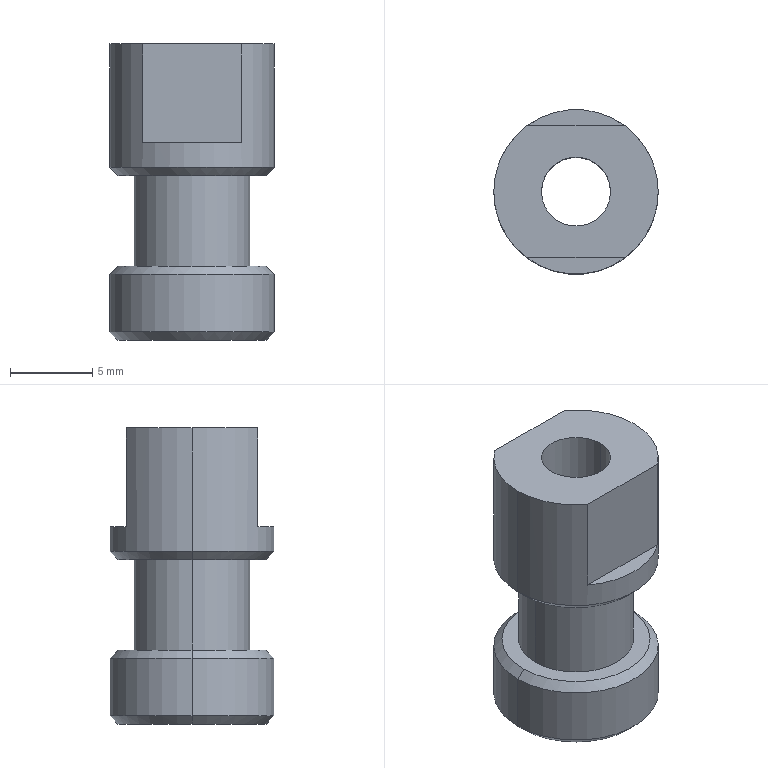Part | STEP file | PN_0051 Mount electronic clip movable connector head | 1 solid | 22 faces | box 10 x 10 x 18 mm | volume 883.594 mm3 | cylinder 8 | plane 8 | cone 6 | commonest cylinder face diameters 10 x4 4.2 x2 7 x2
STEP:
#1=CARTESIAN_POINT('',(0.,0.,0.));
#2=DIRECTION('',(0.,0.,1.));
#3=DIRECTION('',(1.,0.,0.));
#4=AXIS2_PLACEMENT_3D('',#1,#2,#3);
#5=CARTESIAN_POINT('',(-4.5,0.,0.));
#6=VERTEX_POINT('',#5);
#7=CARTESIAN_POINT('',(4.5,0.,0.));
#8=VERTEX_POINT('',#7);
#9=CARTESIAN_POINT('',(0.,0.,0.));
#10=DIRECTION('',(0.,0.,-1.));
#11=DIRECTION('',(1.,0.,0.));
#12=AXIS2_PLACEMENT_3D('',#9,#10,#11);
#13=CIRCLE('',#12,4.5);
#14=CARTESIAN_POINT('',(0.,0.,0.5));
#15=DIRECTION('',(0.,0.,1.));
#16=DIRECTION('',(1.,0.,0.));
#17=AXIS2_PLACEMENT_3D('',#14,#15,#16);
#18=CONICAL_SURFACE('',#17,5.,0.7854);
#19=CARTESIAN_POINT('',(6.283,-0.5));
#20=DIRECTION('',(-1.,0.));
#21=VECTOR('',#20,1.);
#22=LINE('',#19,#21);
#23=(GEOMETRIC_REPRESENTATION_CONTEXT(2)PARAMETRIC_REPRESENTATION_CONTEXT()REPRESENTATION_CONTEXT('',''));
#24=DEFINITIONAL_REPRESENTATION('',(#22),#23);
#25=PCURVE('',#18,#24);
#26=CARTESIAN_POINT('',(0.,0.,0.));
#27=DIRECTION('',(0.,0.,1.));
#28=DIRECTION('',(1.,0.,0.));
#29=AXIS2_PLACEMENT_3D('',#26,#27,#28);
#30=PLANE('',#29);
#31=CARTESIAN_POINT('',(4.5,0.));
#32=CARTESIAN_POINT('',(4.5,-7.794));
#33=CARTESIAN_POINT('',(-2.25,-3.897));
#34=CARTESIAN_POINT('',(-9.,0.));
#35=CARTESIAN_POINT('',(-2.25,3.897));
#36=CARTESIAN_POINT('',(4.5,7.794));
#37=CARTESIAN_POINT('',(4.5,0.));
#38=(BOUNDED_CURVE()B_SPLINE_CURVE(2,(#31,#32,#33,#34,#35,#36,#37),.UNSPECIFIED.,.T.,.F.)B_SPLINE_CURVE_WITH_KNOTS((1,2,2,2,2,1),(-2.094,0.,2.094,4.189,6.283,8.378),.UNSPECIFIED.)CURVE()GEOMETRIC_REPRESENTATION_ITEM()RATIONAL_B_SPLINE_CURVE((1.,0.5,1.,0.5,1.,0.5,1.))REPRESENTATION_ITEM(''));
#39=(GEOMETRIC_REPRESENTATION_CONTEXT(2)PARAMETRIC_REPRESENTATION_CONTEXT()REPRESENTATION_CONTEXT('',''));
#40=DEFINITIONAL_REPRESENTATION('',(#38),#39);
#41=PCURVE('',#30,#40);
#42=SURFACE_CURVE('',#13,(#25,#41),.PCURVE_S1.);
#43=EDGE_CURVE('',#6,#8,#42,.T.);
#44=ORIENTED_EDGE('',*,*,#43,.F.);
#45=CARTESIAN_POINT('',(-5.,0.,0.5));
#46=VERTEX_POINT('',#45);
#47=CARTESIAN_POINT('',(-5.,0.,0.5));
#48=DIRECTION('',(-0.7071,0.,0.7071));
#49=VECTOR('',#48,1.);
#50=LINE('',#47,#49);
#51=CARTESIAN_POINT('',(3.142,0.));
#52=DIRECTION('',(0.,1.));
#53=VECTOR('',#52,1.);
#54=LINE('',#51,#53);
#55=(GEOMETRIC_REPRESENTATION_CONTEXT(2)PARAMETRIC_REPRESENTATION_CONTEXT()REPRESENTATION_CONTEXT('',''));
#56=DEFINITIONAL_REPRESENTATION('',(#54),#55);
#57=PCURVE('',#18,#56);
#58=CARTESIAN_POINT('',(0.,0.,0.5));
#59=DIRECTION('',(0.,0.,1.));
#60=DIRECTION('',(1.,0.,0.));
#61=AXIS2_PLACEMENT_3D('',#58,#59,#60);
#62=CONICAL_SURFACE('',#61,5.,0.7854);
#63=CARTESIAN_POINT('',(3.142,0.));
#64=DIRECTION('',(0.,1.));
#65=VECTOR('',#64,1.);
#66=LINE('',#63,#65);
#67=(GEOMETRIC_REPRESENTATION_CONTEXT(2)PARAMETRIC_REPRESENTATION_CONTEXT()REPRESENTATION_CONTEXT('',''));
#68=DEFINITIONAL_REPRESENTATION('',(#66),#67);
#69=PCURVE('',#62,#68);
#70=SURFACE_CURVE('',#50,(#57,#69),.PCURVE_S1.);
#71=EDGE_CURVE('',#6,#46,#70,.T.);
#72=ORIENTED_EDGE('',*,*,#71,.T.);
#73=CARTESIAN_POINT('',(5.,0.,0.5));
#74=VERTEX_POINT('',#73);
#75=CARTESIAN_POINT('',(0.,0.,0.5));
#76=DIRECTION('',(0.,0.,1.));
#77=DIRECTION('',(1.,0.,0.));
#78=AXIS2_PLACEMENT_3D('',#75,#76,#77);
#79=CIRCLE('',#78,5.);
#80=CARTESIAN_POINT('',(0.,0.));
#81=DIRECTION('',(1.,0.));
#82=VECTOR('',#81,1.);
#83=LINE('',#80,#82);
#84=(GEOMETRIC_REPRESENTATION_CONTEXT(2)PARAMETRIC_REPRESENTATION_CONTEXT()REPRESENTATION_CONTEXT('',''));
#85=DEFINITIONAL_REPRESENTATION('',(#83),#84);
#86=PCURVE('',#18,#85);
#87=CARTESIAN_POINT('',(0.,0.,4.5));
#88=DIRECTION('',(0.,0.,-1.));
#89=DIRECTION('',(-1.,0.,0.));
#90=AXIS2_PLACEMENT_3D('',#87,#88,#89);
#91=CYLINDRICAL_SURFACE('',#90,5.);
#92=CARTESIAN_POINT('',(3.142,4.));
#93=DIRECTION('',(-1.,0.));
#94=VECTOR('',#93,1.);
#95=LINE('',#92,#94);
#96=(GEOMETRIC_REPRESENTATION_CONTEXT(2)PARAMETRIC_REPRESENTATION_CONTEXT()REPRESENTATION_CONTEXT('',''));
#97=DEFINITIONAL_REPRESENTATION('',(#95),#96);
#98=PCURVE('',#91,#97);
#99=SURFACE_CURVE('',#79,(#86,#98),.PCURVE_S1.);
#100=EDGE_CURVE('',#74,#46,#99,.T.);
#101=ORIENTED_EDGE('',*,*,#100,.F.);
#102=CARTESIAN_POINT('',(5.,0.,0.5));
#103=DIRECTION('',(0.7071,0.,0.7071));
#104=VECTOR('',#103,1.);
#105=LINE('',#102,#104);
#106=CARTESIAN_POINT('',(0.,0.));
#107=DIRECTION('',(0.,1.));
#108=VECTOR('',#107,1.);
#109=LINE('',#106,#108);
#110=(GEOMETRIC_REPRESENTATION_CONTEXT(2)PARAMETRIC_REPRESENTATION_CONTEXT()REPRESENTATION_CONTEXT('',''));
#111=DEFINITIONAL_REPRESENTATION('',(#109),#110);
#112=PCURVE('',#18,#111);
#113=CARTESIAN_POINT('',(6.283,0.));
#114=DIRECTION('',(0.,1.));
#115=VECTOR('',#114,1.);
#116=LINE('',#113,#115);
#117=(GEOMETRIC_REPRESENTATION_CONTEXT(2)PARAMETRIC_REPRESENTATION_CONTEXT()REPRESENTATION_CONTEXT('',''));
#118=DEFINITIONAL_REPRESENTATION('',(#116),#117);
#119=PCURVE('',#62,#118);
#120=SURFACE_CURVE('',#105,(#112,#119),.PCURVE_S1.);
#121=EDGE_CURVE('',#8,#74,#120,.T.);
#122=ORIENTED_EDGE('',*,*,#121,.F.);
#123=EDGE_LOOP('',(#44,#72,#101,#122));
#124=FACE_BOUND('',#123,.T.);
#125=ADVANCED_FACE('',(#124),#18,.T.);
#126=CARTESIAN_POINT('',(4.5,0.,4.5));
#127=VERTEX_POINT('',#126);
#128=CARTESIAN_POINT('',(-4.5,0.,4.5));
#129=VERTEX_POINT('',#128);
#130=CARTESIAN_POINT('',(0.,0.,4.5));
#131=DIRECTION('',(0.,0.,1.));
#132=DIRECTION('',(1.,0.,0.));
#133=AXIS2_PLACEMENT_3D('',#130,#131,#132);
#134=CIRCLE('',#133,4.5);
#135=CARTESIAN_POINT('',(0.,0.,4.5));
#136=DIRECTION('',(0.,0.,-1.));
#137=DIRECTION('',(-1.,0.,0.));
#138=AXIS2_PLACEMENT_3D('',#135,#136,#137);
#139=CONICAL_SURFACE('',#138,4.5,0.7854);
#140=CARTESIAN_POINT('',(3.142,0.));
#141=DIRECTION('',(-1.,0.));
#142=VECTOR('',#141,1.);
#143=LINE('',#140,#142);
#144=(GEOMETRIC_REPRESENTATION_CONTEXT(2)PARAMETRIC_REPRESENTATION_CONTEXT()REPRESENTATION_CONTEXT('',''));
#145=DEFINITIONAL_REPRESENTATION('',(#143),#144);
#146=PCURVE('',#139,#145);
#147=CARTESIAN_POINT('',(0.,0.,4.5));
#148=DIRECTION('',(0.,0.,1.));
#149=DIRECTION('',(1.,0.,0.));
#150=AXIS2_PLACEMENT_3D('',#147,#148,#149);
#151=PLANE('',#150);
#152=CARTESIAN_POINT('',(0.,0.));
#153=DIRECTION('',(1.,0.));
#154=AXIS2_PLACEMENT_2D('',#152,#153);
#155=CIRCLE('',#154,4.5);
#156=(GEOMETRIC_REPRESENTATION_CONTEXT(2)PARAMETRIC_REPRESENTATION_CONTEXT()REPRESENTATION_CONTEXT('',''));
#157=DEFINITIONAL_REPRESENTATION('',(#155),#156);
#158=PCURVE('',#151,#157);
#159=SURFACE_CURVE('',#134,(#146,#158),.PCURVE_S1.);
#160=EDGE_CURVE('',#127,#129,#159,.T.);
#161=ORIENTED_EDGE('',*,*,#160,.F.);
#162=CARTESIAN_POINT('',(5.,0.,4.));
#163=VERTEX_POINT('',#162);
#164=CARTESIAN_POINT('',(4.5,0.,4.5));
#165=DIRECTION('',(0.7071,0.,-0.7071));
#166=VECTOR('',#165,1.);
#167=LINE('',#164,#166);
#168=CARTESIAN_POINT('',(3.142,0.));
#169=DIRECTION('',(0.,1.));
#170=VECTOR('',#169,1.);
#171=LINE('',#168,#170);
#172=(GEOMETRIC_REPRESENTATION_CONTEXT(2)PARAMETRIC_REPRESENTATION_CONTEXT()REPRESENTATION_CONTEXT('',''));
#173=DEFINITIONAL_REPRESENTATION('',(#171),#172);
#174=PCURVE('',#139,#173);
#175=CARTESIAN_POINT('',(0.,0.,4.5));
#176=DIRECTION('',(0.,0.,-1.));
#177=DIRECTION('',(-1.,0.,0.));
#178=AXIS2_PLACEMENT_3D('',#175,#176,#177);
#179=CONICAL_SURFACE('',#178,4.5,0.7854);
#180=CARTESIAN_POINT('',(3.142,0.));
#181=DIRECTION('',(0.,1.));
#182=VECTOR('',#181,1.);
#183=LINE('',#180,#182);
#184=(GEOMETRIC_REPRESENTATION_CONTEXT(2)PARAMETRIC_REPRESENTATION_CONTEXT()REPRESENTATION_CONTEXT('',''));
#185=DEFINITIONAL_REPRESENTATION('',(#183),#184);
#186=PCURVE('',#179,#185);
#187=SURFACE_CURVE('',#167,(#174,#186),.PCURVE_S1.);
#188=EDGE_CURVE('',#127,#163,#187,.T.);
#189=ORIENTED_EDGE('',*,*,#188,.T.);
#190=CARTESIAN_POINT('',(-5.,0.,4.));
#191=VERTEX_POINT('',#190);
#192=CARTESIAN_POINT('',(0.,0.,4.));
#193=DIRECTION('',(0.,0.,-1.));
#194=DIRECTION('',(1.,0.,0.));
#195=AXIS2_PLACEMENT_3D('',#192,#193,#194);
#196=CIRCLE('',#195,5.);
#197=CARTESIAN_POINT('',(-3.142,0.5));
#198=DIRECTION('',(1.,0.));
#199=VECTOR('',#198,1.);
#200=LINE('',#197,#199);
#201=(GEOMETRIC_REPRESENTATION_CONTEXT(2)PARAMETRIC_REPRESENTATION_CONTEXT()REPRESENTATION_CONTEXT('',''));
#202=DEFINITIONAL_REPRESENTATION('',(#200),#201);
#203=PCURVE('',#139,#202);
#204=CARTESIAN_POINT('',(-3.142,0.5));
#205=DIRECTION('',(1.,0.));
#206=VECTOR('',#205,1.);
#207=LINE('',#204,#206);
#208=(GEOMETRIC_REPRESENTATION_CONTEXT(2)PARAMETRIC_REPRESENTATION_CONTEXT()REPRESENTATION_CONTEXT('',''));
#209=DEFINITIONAL_REPRESENTATION('',(#207),#208);
#210=PCURVE('',#91,#209);
#211=SURFACE_CURVE('',#196,(#203,#210),.PCURVE_S1.);
#212=EDGE_CURVE('',#191,#163,#211,.T.);
#213=ORIENTED_EDGE('',*,*,#212,.F.);
#214=CARTESIAN_POINT('',(-4.5,0.,4.5));
#215=DIRECTION('',(-0.7071,0.,-0.7071));
#216=VECTOR('',#215,1.);
#217=LINE('',#214,#216);
#218=CARTESIAN_POINT('',(0.,0.));
#219=DIRECTION('',(0.,1.));
#220=VECTOR('',#219,1.);
#221=LINE('',#218,#220);
#222=(GEOMETRIC_REPRESENTATION_CONTEXT(2)PARAMETRIC_REPRESENTATION_CONTEXT()REPRESENTATION_CONTEXT('',''));
#223=DEFINITIONAL_REPRESENTATION('',(#221),#222);
#224=PCURVE('',#139,#223);
#225=CARTESIAN_POINT('',(6.283,0.));
#226=DIRECTION('',(0.,1.));
#227=VECTOR('',#226,1.);
#228=LINE('',#225,#227);
#229=(GEOMETRIC_REPRESENTATION_CONTEXT(2)PARAMETRIC_REPRESENTATION_CONTEXT()REPRESENTATION_CONTEXT('',''));
#230=DEFINITIONAL_REPRESENTATION('',(#228),#229);
#231=PCURVE('',#179,#230);
#232=SURFACE_CURVE('',#217,(#224,#231),.PCURVE_S1.);
#233=EDGE_CURVE('',#129,#191,#232,.T.);
#234=ORIENTED_EDGE('',*,*,#233,.F.);
#235=EDGE_LOOP('',(#161,#189,#213,#234));
#236=FACE_BOUND('',#235,.T.);
#237=ADVANCED_FACE('',(#236),#139,.T.);
#238=CARTESIAN_POINT('',(-4.5,0.,10.));
#239=VERTEX_POINT('',#238);
#240=CARTESIAN_POINT('',(4.5,0.,10.));
#241=VERTEX_POINT('',#240);
#242=CARTESIAN_POINT('',(0.,0.,10.));
#243=DIRECTION('',(0.,0.,-1.));
#244=DIRECTION('',(1.,0.,0.));
#245=AXIS2_PLACEMENT_3D('',#242,#243,#244);
#246=CIRCLE('',#245,4.5);
#247=CARTESIAN_POINT('',(0.,0.,10.5));
#248=DIRECTION('',(0.,0.,1.));
#249=DIRECTION('',(1.,0.,0.));
#250=AXIS2_PLACEMENT_3D('',#247,#248,#249);
#251=CONICAL_SURFACE('',#250,5.,0.7854);
#252=CARTESIAN_POINT('',(6.283,-0.5));
#253=DIRECTION('',(-1.,0.));
#254=VECTOR('',#253,1.);
#255=LINE('',#252,#254);
#256=(GEOMETRIC_REPRESENTATION_CONTEXT(2)PARAMETRIC_REPRESENTATION_CONTEXT()REPRESENTATION_CONTEXT('',''));
#257=DEFINITIONAL_REPRESENTATION('',(#255),#256);
#258=PCURVE('',#251,#257);
#259=CARTESIAN_POINT('',(0.,0.,10.));
#260=DIRECTION('',(0.,0.,1.));
#261=DIRECTION('',(1.,0.,0.));
#262=AXIS2_PLACEMENT_3D('',#259,#260,#261);
#263=PLANE('',#262);
#264=CARTESIAN_POINT('',(4.5,0.));
#265=CARTESIAN_POINT('',(4.5,-7.794));
#266=CARTESIAN_POINT('',(-2.25,-3.897));
#267=CARTESIAN_POINT('',(-9.,0.));
#268=CARTESIAN_POINT('',(-2.25,3.897));
#269=CARTESIAN_POINT('',(4.5,7.794));
#270=CARTESIAN_POINT('',(4.5,0.));
#271=(BOUNDED_CURVE()B_SPLINE_CURVE(2,(#264,#265,#266,#267,#268,#269,#270),.UNSPECIFIED.,.T.,.F.)B_SPLINE_CURVE_WITH_KNOTS((1,2,2,2,2,1),(-2.094,0.,2.094,4.189,6.283,8.378),.UNSPECIFIED.)CURVE()GEOMETRIC_REPRESENTATION_ITEM()RATIONAL_B_SPLINE_CURVE((1.,0.5,1.,0.5,1.,0.5,1.))REPRESENTATION_ITEM(''));
#272=(GEOMETRIC_REPRESENTATION_CONTEXT(2)PARAMETRIC_REPRESENTATION_CONTEXT()REPRESENTATION_CONTEXT('',''));
#273=DEFINITIONAL_REPRESENTATION('',(#271),#272);
#274=PCURVE('',#263,#273);
#275=SURFACE_CURVE('',#246,(#258,#274),.PCURVE_S1.);
#276=EDGE_CURVE('',#239,#241,#275,.T.);
#277=ORIENTED_EDGE('',*,*,#276,.F.);
#278=CARTESIAN_POINT('',(-5.,0.,10.5));
#279=VERTEX_POINT('',#278);
#280=CARTESIAN_POINT('',(-5.,0.,10.5));
#281=DIRECTION('',(-0.7071,0.,0.7071));
#282=VECTOR('',#281,1.);
#283=LINE('',#280,#282);
#284=CARTESIAN_POINT('',(3.142,0.));
#285=DIRECTION('',(0.,1.));
#286=VECTOR('',#285,1.);
#287=LINE('',#284,#286);
#288=(GEOMETRIC_REPRESENTATION_CONTEXT(2)PARAMETRIC_REPRESENTATION_CONTEXT()REPRESENTATION_CONTEXT('',''));
#289=DEFINITIONAL_REPRESENTATION('',(#287),#288);
#290=PCURVE('',#251,#289);
#291=CARTESIAN_POINT('',(0.,0.,10.5));
#292=DIRECTION('',(0.,0.,1.));
#293=DIRECTION('',(1.,0.,0.));
#294=AXIS2_PLACEMENT_3D('',#291,#292,#293);
#295=CONICAL_SURFACE('',#294,5.,0.7854);
#296=CARTESIAN_POINT('',(3.142,0.));
#297=DIRECTION('',(0.,1.));
#298=VECTOR('',#297,1.);
#299=LINE('',#296,#298);
#300=(GEOMETRIC_REPRESENTATION_CONTEXT(2)PARAMETRIC_REPRESENTATION_CONTEXT()REPRESENTATION_CONTEXT('',''));
#301=DEFINITIONAL_REPRESENTATION('',(#299),#300);
#302=PCURVE('',#295,#301);
#303=SURFACE_CURVE('',#283,(#290,#302),.PCURVE_S1.);
#304=EDGE_CURVE('',#239,#279,#303,.T.);
#305=ORIENTED_EDGE('',*,*,#304,.T.);
#306=CARTESIAN_POINT('',(5.,0.,10.5));
#307=VERTEX_POINT('',#306);
#308=CARTESIAN_POINT('',(0.,0.,10.5));
#309=DIRECTION('',(0.,0.,1.));
#310=DIRECTION('',(1.,0.,0.));
#311=AXIS2_PLACEMENT_3D('',#308,#309,#310);
#312=CIRCLE('',#311,5.);
#313=CARTESIAN_POINT('',(0.,0.));
#314=DIRECTION('',(1.,0.));
#315=VECTOR('',#314,1.);
#316=LINE('',#313,#315);
#317=(GEOMETRIC_REPRESENTATION_CONTEXT(2)PARAMETRIC_REPRESENTATION_CONTEXT()REPRESENTATION_CONTEXT('',''));
#318=DEFINITIONAL_REPRESENTATION('',(#316),#317);
#319=PCURVE('',#251,#318);
#320=CARTESIAN_POINT('',(0.,0.,18.));
#321=DIRECTION('',(0.,0.,-1.));
#322=DIRECTION('',(-1.,0.,0.));
#323=AXIS2_PLACEMENT_3D('',#320,#321,#322);
#324=CYLINDRICAL_SURFACE('',#323,5.);
#325=CARTESIAN_POINT('',(3.142,7.5));
#326=DIRECTION('',(-1.,0.));
#327=VECTOR('',#326,1.);
#328=LINE('',#325,#327);
#329=(GEOMETRIC_REPRESENTATION_CONTEXT(2)PARAMETRIC_REPRESENTATION_CONTEXT()REPRESENTATION_CONTEXT('',''));
#330=DEFINITIONAL_REPRESENTATION('',(#328),#329);
#331=PCURVE('',#324,#330);
#332=SURFACE_CURVE('',#312,(#319,#331),.PCURVE_S1.);
#333=EDGE_CURVE('',#307,#279,#332,.T.);
#334=ORIENTED_EDGE('',*,*,#333,.F.);
#335=CARTESIAN_POINT('',(5.,0.,10.5));
#336=DIRECTION('',(0.7071,0.,0.7071));
#337=VECTOR('',#336,1.);
#338=LINE('',#335,#337);
#339=CARTESIAN_POINT('',(0.,0.));
#340=DIRECTION('',(0.,1.));
#341=VECTOR('',#340,1.);
#342=LINE('',#339,#341);
#343=(GEOMETRIC_REPRESENTATION_CONTEXT(2)PARAMETRIC_REPRESENTATION_CONTEXT()REPRESENTATION_CONTEXT('',''));
#344=DEFINITIONAL_REPRESENTATION('',(#342),#343);
#345=PCURVE('',#251,#344);
#346=CARTESIAN_POINT('',(6.283,0.));
#347=DIRECTION('',(0.,1.));
#348=VECTOR('',#347,1.);
#349=LINE('',#346,#348);
#350=(GEOMETRIC_REPRESENTATION_CONTEXT(2)PARAMETRIC_REPRESENTATION_CONTEXT()REPRESENTATION_CONTEXT('',''));
#351=DEFINITIONAL_REPRESENTATION('',(#349),#350);
#352=PCURVE('',#295,#351);
#353=SURFACE_CURVE('',#338,(#345,#352),.PCURVE_S1.);
#354=EDGE_CURVE('',#241,#307,#353,.T.);
#355=ORIENTED_EDGE('',*,*,#354,.F.);
#356=EDGE_LOOP('',(#277,#305,#334,#355));
#357=FACE_BOUND('',#356,.T.);
#358=ADVANCED_FACE('',(#357),#251,.T.);
#359=CARTESIAN_POINT('',(2.1,0.,0.));
#360=VERTEX_POINT('',#359);
#361=CARTESIAN_POINT('',(2.1,0.,18.));
#362=VERTEX_POINT('',#361);
#363=CARTESIAN_POINT('',(2.1,0.,18.));
#364=DIRECTION('',(0.,0.,1.));
#365=VECTOR('',#364,1.);
#366=LINE('',#363,#365);
#367=CARTESIAN_POINT('',(0.,0.,18.));
#368=DIRECTION('',(0.,0.,1.));
#369=DIRECTION('',(1.,0.,0.));
#370=AXIS2_PLACEMENT_3D('',#367,#368,#369);
#371=CYLINDRICAL_SURFACE('',#370,2.1);
#372=CARTESIAN_POINT('',(6.283,0.));
#373=DIRECTION('',(0.,1.));
#374=VECTOR('',#373,1.);
#375=LINE('',#372,#374);
#376=(GEOMETRIC_REPRESENTATION_CONTEXT(2)PARAMETRIC_REPRESENTATION_CONTEXT()REPRESENTATION_CONTEXT('',''));
#377=DEFINITIONAL_REPRESENTATION('',(#375),#376);
#378=PCURVE('',#371,#377);
#379=CARTESIAN_POINT('',(0.,0.,18.));
#380=DIRECTION('',(0.,0.,1.));
#381=DIRECTION('',(1.,0.,0.));
#382=AXIS2_PLACEMENT_3D('',#379,#380,#381);
#383=CYLINDRICAL_SURFACE('',#382,2.1);
#384=CARTESIAN_POINT('',(0.,0.));
#385=DIRECTION('',(0.,1.));
#386=VECTOR('',#385,1.);
#387=LINE('',#384,#386);
#388=(GEOMETRIC_REPRESENTATION_CONTEXT(2)PARAMETRIC_REPRESENTATION_CONTEXT()REPRESENTATION_CONTEXT('',''));
#389=DEFINITIONAL_REPRESENTATION('',(#387),#388);
#390=PCURVE('',#383,#389);
#391=SURFACE_CURVE('',#366,(#378,#390),.PCURVE_S1.);
#392=EDGE_CURVE('',#360,#362,#391,.T.);
#393=ORIENTED_EDGE('',*,*,#392,.T.);
#394=CARTESIAN_POINT('',(-2.1,0.,18.));
#395=VERTEX_POINT('',#394);
#396=CARTESIAN_POINT('',(0.,0.,18.));
#397=DIRECTION('',(0.,0.,1.));
#398=DIRECTION('',(1.,0.,0.));
#399=AXIS2_PLACEMENT_3D('',#396,#397,#398);
#400=CIRCLE('',#399,2.1);
#401=CARTESIAN_POINT('',(0.,0.));
#402=DIRECTION('',(1.,0.));
#403=VECTOR('',#402,1.);
#404=LINE('',#401,#403);
#405=(GEOMETRIC_REPRESENTATION_CONTEXT(2)PARAMETRIC_REPRESENTATION_CONTEXT()REPRESENTATION_CONTEXT('',''));
#406=DEFINITIONAL_REPRESENTATION('',(#404),#405);
#407=PCURVE('',#371,#406);
#408=CARTESIAN_POINT('',(0.,0.,18.));
#409=DIRECTION('',(0.,0.,1.));
#410=DIRECTION('',(1.,0.,0.));
#411=AXIS2_PLACEMENT_3D('',#408,#409,#410);
#412=PLANE('',#411);
#413=CARTESIAN_POINT('',(0.,0.));
#414=DIRECTION('',(1.,0.));
#415=AXIS2_PLACEMENT_2D('',#413,#414);
#416=CIRCLE('',#415,2.1);
#417=(GEOMETRIC_REPRESENTATION_CONTEXT(2)PARAMETRIC_REPRESENTATION_CONTEXT()REPRESENTATION_CONTEXT('',''));
#418=DEFINITIONAL_REPRESENTATION('',(#416),#417);
#419=PCURVE('',#412,#418);
#420=SURFACE_CURVE('',#400,(#407,#419),.PCURVE_S1.);
#421=EDGE_CURVE('',#395,#362,#420,.T.);
#422=ORIENTED_EDGE('',*,*,#421,.F.);
#423=CARTESIAN_POINT('',(-2.1,0.,0.));
#424=VERTEX_POINT('',#423);
#425=CARTESIAN_POINT('',(-2.1,0.,18.));
#426=DIRECTION('',(0.,0.,1.));
#427=VECTOR('',#426,1.);
#428=LINE('',#425,#427);
#429=CARTESIAN_POINT('',(3.142,0.));
#430=DIRECTION('',(0.,1.));
#431=VECTOR('',#430,1.);
#432=LINE('',#429,#431);
#433=(GEOMETRIC_REPRESENTATION_CONTEXT(2)PARAMETRIC_REPRESENTATION_CONTEXT()REPRESENTATION_CONTEXT('',''));
#434=DEFINITIONAL_REPRESENTATION('',(#432),#433);
#435=PCURVE('',#371,#434);
#436=CARTESIAN_POINT('',(3.142,0.));
#437=DIRECTION('',(0.,1.));
#438=VECTOR('',#437,1.);
#439=LINE('',#436,#438);
#440=(GEOMETRIC_REPRESENTATION_CONTEXT(2)PARAMETRIC_REPRESENTATION_CONTEXT()REPRESENTATION_CONTEXT('',''));
#441=DEFINITIONAL_REPRESENTATION('',(#439),#440);
#442=PCURVE('',#383,#441);
#443=SURFACE_CURVE('',#428,(#435,#442),.PCURVE_S1.);
#444=EDGE_CURVE('',#424,#395,#443,.T.);
#445=ORIENTED_EDGE('',*,*,#444,.F.);
#446=CARTESIAN_POINT('',(0.,0.,0.));
#447=DIRECTION('',(0.,0.,1.));
#448=DIRECTION('',(1.,0.,0.));
#449=AXIS2_PLACEMENT_3D('',#446,#447,#448);
#450=CIRCLE('',#449,2.1);
#451=CARTESIAN_POINT('',(0.,-18.));
#452=DIRECTION('',(1.,0.));
#453=VECTOR('',#452,1.);
#454=LINE('',#451,#453);
#455=(GEOMETRIC_REPRESENTATION_CONTEXT(2)PARAMETRIC_REPRESENTATION_CONTEXT()REPRESENTATION_CONTEXT('',''));
#456=DEFINITIONAL_REPRESENTATION('',(#454),#455);
#457=PCURVE('',#371,#456);
#458=CARTESIAN_POINT('',(0.,0.));
#459=DIRECTION('',(1.,0.));
#460=AXIS2_PLACEMENT_2D('',#458,#459);
#461=CIRCLE('',#460,2.1);
#462=(GEOMETRIC_REPRESENTATION_CONTEXT(2)PARAMETRIC_REPRESENTATION_CONTEXT()REPRESENTATION_CONTEXT('',''));
#463=DEFINITIONAL_REPRESENTATION('',(#461),#462);
#464=PCURVE('',#30,#463);
#465=SURFACE_CURVE('',#450,(#457,#464),.PCURVE_S1.);
#466=EDGE_CURVE('',#424,#360,#465,.T.);
#467=ORIENTED_EDGE('',*,*,#466,.T.);
#468=EDGE_LOOP('',(#393,#422,#445,#467));
#469=FACE_BOUND('',#468,.F.);
#470=ADVANCED_FACE('',(#469),#371,.F.);
#471=CARTESIAN_POINT('',(5.,0.,18.));
#472=VERTEX_POINT('',#471);
#473=CARTESIAN_POINT('',(3.,4.,18.));
#474=VERTEX_POINT('',#473);
#475=CARTESIAN_POINT('',(0.,0.,18.));
#476=DIRECTION('',(0.,0.,1.));
#477=DIRECTION('',(1.,0.,0.));
#478=AXIS2_PLACEMENT_3D('',#475,#476,#477);
#479=CIRCLE('',#478,5.);
#480=CARTESIAN_POINT('',(3.142,0.));
#481=DIRECTION('',(-1.,0.));
#482=VECTOR('',#481,1.);
#483=LINE('',#480,#482);
#484=(GEOMETRIC_REPRESENTATION_CONTEXT(2)PARAMETRIC_REPRESENTATION_CONTEXT()REPRESENTATION_CONTEXT('',''));
#485=DEFINITIONAL_REPRESENTATION('',(#483),#484);
#486=PCURVE('',#324,#485);
#487=CARTESIAN_POINT('',(0.,0.));
#488=DIRECTION('',(1.,0.));
#489=AXIS2_PLACEMENT_2D('',#487,#488);
#490=CIRCLE('',#489,5.);
#491=(GEOMETRIC_REPRESENTATION_CONTEXT(2)PARAMETRIC_REPRESENTATION_CONTEXT()REPRESENTATION_CONTEXT('',''));
#492=DEFINITIONAL_REPRESENTATION('',(#490),#491);
#493=PCURVE('',#412,#492);
#494=SURFACE_CURVE('',#479,(#486,#493),.PCURVE_S1.);
#495=EDGE_CURVE('',#472,#474,#494,.T.);
#496=ORIENTED_EDGE('',*,*,#495,.F.);
#497=CARTESIAN_POINT('',(5.,0.,18.));
#498=DIRECTION('',(0.,0.,-1.));
#499=VECTOR('',#498,1.);
#500=LINE('',#497,#499);
#501=CARTESIAN_POINT('',(3.142,0.));
#502=DIRECTION('',(0.,1.));
#503=VECTOR('',#502,1.);
#504=LINE('',#501,#503);
#505=(GEOMETRIC_REPRESENTATION_CONTEXT(2)PARAMETRIC_REPRESENTATION_CONTEXT()REPRESENTATION_CONTEXT('',''));
#506=DEFINITIONAL_REPRESENTATION('',(#504),#505);
#507=PCURVE('',#324,#506);
#508=CARTESIAN_POINT('',(0.,0.,18.));
#509=DIRECTION('',(0.,0.,-1.));
#510=DIRECTION('',(-1.,0.,0.));
#511=AXIS2_PLACEMENT_3D('',#508,#509,#510);
#512=CYLINDRICAL_SURFACE('',#511,5.);
#513=CARTESIAN_POINT('',(3.142,0.));
#514=DIRECTION('',(0.,1.));
#515=VECTOR('',#514,1.);
#516=LINE('',#513,#515);
#517=(GEOMETRIC_REPRESENTATION_CONTEXT(2)PARAMETRIC_REPRESENTATION_CONTEXT()REPRESENTATION_CONTEXT('',''));
#518=DEFINITIONAL_REPRESENTATION('',(#516),#517);
#519=PCURVE('',#512,#518);
#520=SURFACE_CURVE('',#500,(#507,#519),.PCURVE_S1.);
#521=EDGE_CURVE('',#472,#307,#520,.T.);
#522=ORIENTED_EDGE('',*,*,#521,.T.);
#523=ORIENTED_EDGE('',*,*,#333,.T.);
#524=CARTESIAN_POINT('',(-5.,0.,18.));
#525=VERTEX_POINT('',#524);
#526=CARTESIAN_POINT('',(-5.,0.,18.));
#527=DIRECTION('',(0.,0.,-1.));
#528=VECTOR('',#527,1.);
#529=LINE('',#526,#528);
#530=CARTESIAN_POINT('',(0.,0.));
#531=DIRECTION('',(0.,1.));
#532=VECTOR('',#531,1.);
#533=LINE('',#530,#532);
#534=(GEOMETRIC_REPRESENTATION_CONTEXT(2)PARAMETRIC_REPRESENTATION_CONTEXT()REPRESENTATION_CONTEXT('',''));
#535=DEFINITIONAL_REPRESENTATION('',(#533),#534);
#536=PCURVE('',#324,#535);
#537=CARTESIAN_POINT('',(6.283,0.));
#538=DIRECTION('',(0.,1.));
#539=VECTOR('',#538,1.);
#540=LINE('',#537,#539);
#541=(GEOMETRIC_REPRESENTATION_CONTEXT(2)PARAMETRIC_REPRESENTATION_CONTEXT()REPRESENTATION_CONTEXT('',''));
#542=DEFINITIONAL_REPRESENTATION('',(#540),#541);
#543=PCURVE('',#512,#542);
#544=SURFACE_CURVE('',#529,(#536,#543),.PCURVE_S1.);
#545=EDGE_CURVE('',#525,#279,#544,.T.);
#546=ORIENTED_EDGE('',*,*,#545,.F.);
#547=CARTESIAN_POINT('',(-3.,4.,18.));
#548=VERTEX_POINT('',#547);
#549=CARTESIAN_POINT('',(0.,0.,18.));
#550=DIRECTION('',(0.,0.,1.));
#551=DIRECTION('',(1.,0.,0.));
#552=AXIS2_PLACEMENT_3D('',#549,#550,#551);
#553=CIRCLE('',#552,5.);
#554=CARTESIAN_POINT('',(3.142,0.));
#555=DIRECTION('',(-1.,0.));
#556=VECTOR('',#555,1.);
#557=LINE('',#554,#556);
#558=(GEOMETRIC_REPRESENTATION_CONTEXT(2)PARAMETRIC_REPRESENTATION_CONTEXT()REPRESENTATION_CONTEXT('',''));
#559=DEFINITIONAL_REPRESENTATION('',(#557),#558);
#560=PCURVE('',#324,#559);
#561=CARTESIAN_POINT('',(0.,0.));
#562=DIRECTION('',(1.,0.));
#563=AXIS2_PLACEMENT_2D('',#561,#562);
#564=CIRCLE('',#563,5.);
#565=(GEOMETRIC_REPRESENTATION_CONTEXT(2)PARAMETRIC_REPRESENTATION_CONTEXT()REPRESENTATION_CONTEXT('',''));
#566=DEFINITIONAL_REPRESENTATION('',(#564),#565);
#567=PCURVE('',#412,#566);
#568=SURFACE_CURVE('',#553,(#560,#567),.PCURVE_S1.);
#569=EDGE_CURVE('',#548,#525,#568,.T.);
#570=ORIENTED_EDGE('',*,*,#569,.F.);
#571=CARTESIAN_POINT('',(-3.,4.,12.));
#572=VERTEX_POINT('',#571);
#573=CARTESIAN_POINT('',(-3.,4.,18.));
#574=DIRECTION('',(0.,0.,-1.));
#575=VECTOR('',#574,1.);
#576=LINE('',#573,#575);
#577=CARTESIAN_POINT('',(0.9273,0.));
#578=DIRECTION('',(0.,1.));
#579=VECTOR('',#578,1.);
#580=LINE('',#577,#579);
#581=(GEOMETRIC_REPRESENTATION_CONTEXT(2)PARAMETRIC_REPRESENTATION_CONTEXT()REPRESENTATION_CONTEXT('',''));
#582=DEFINITIONAL_REPRESENTATION('',(#580),#581);
#583=PCURVE('',#324,#582);
#584=CARTESIAN_POINT('',(5.719,4.,12.));
#585=DIRECTION('',(0.,-1.,0.));
#586=DIRECTION('',(1.,0.,0.));
#587=AXIS2_PLACEMENT_3D('',#584,#585,#586);
#588=PLANE('',#587);
#589=CARTESIAN_POINT('',(-8.719,6.));
#590=DIRECTION('',(0.,-1.));
#591=VECTOR('',#590,1.);
#592=LINE('',#589,#591);
#593=(GEOMETRIC_REPRESENTATION_CONTEXT(2)PARAMETRIC_REPRESENTATION_CONTEXT()REPRESENTATION_CONTEXT('',''));
#594=DEFINITIONAL_REPRESENTATION('',(#592),#593);
#595=PCURVE('',#588,#594);
#596=SURFACE_CURVE('',#576,(#583,#595),.PCURVE_S1.);
#597=EDGE_CURVE('',#548,#572,#596,.T.);
#598=ORIENTED_EDGE('',*,*,#597,.T.);
#599=CARTESIAN_POINT('',(3.,4.,12.));
#600=VERTEX_POINT('',#599);
#601=CARTESIAN_POINT('',(0.,0.,12.));
#602=DIRECTION('',(0.,0.,1.));
#603=DIRECTION('',(1.,0.,0.));
#604=AXIS2_PLACEMENT_3D('',#601,#602,#603);
#605=CIRCLE('',#604,5.);
#606=CARTESIAN_POINT('',(3.142,6.));
#607=DIRECTION('',(-1.,0.));
#608=VECTOR('',#607,1.);
#609=LINE('',#606,#608);
#610=(GEOMETRIC_REPRESENTATION_CONTEXT(2)PARAMETRIC_REPRESENTATION_CONTEXT()REPRESENTATION_CONTEXT('',''));
#611=DEFINITIONAL_REPRESENTATION('',(#609),#610);
#612=PCURVE('',#324,#611);
#613=CARTESIAN_POINT('',(0.,0.,12.));
#614=DIRECTION('',(0.,0.,1.));
#615=DIRECTION('',(1.,0.,0.));
#616=AXIS2_PLACEMENT_3D('',#613,#614,#615);
#617=PLANE('',#616);
#618=CARTESIAN_POINT('',(0.,0.));
#619=DIRECTION('',(1.,0.));
#620=AXIS2_PLACEMENT_2D('',#618,#619);
#621=CIRCLE('',#620,5.);
#622=(GEOMETRIC_REPRESENTATION_CONTEXT(2)PARAMETRIC_REPRESENTATION_CONTEXT()REPRESENTATION_CONTEXT('',''));
#623=DEFINITIONAL_REPRESENTATION('',(#621),#622);
#624=PCURVE('',#617,#623);
#625=SURFACE_CURVE('',#605,(#612,#624),.PCURVE_S1.);
#626=EDGE_CURVE('',#600,#572,#625,.T.);
#627=ORIENTED_EDGE('',*,*,#626,.F.);
#628=CARTESIAN_POINT('',(3.,4.,18.));
#629=DIRECTION('',(0.,0.,1.));
#630=VECTOR('',#629,1.);
#631=LINE('',#628,#630);
#632=CARTESIAN_POINT('',(2.214,0.));
#633=DIRECTION('',(0.,-1.));
#634=VECTOR('',#633,1.);
#635=LINE('',#632,#634);
#636=(GEOMETRIC_REPRESENTATION_CONTEXT(2)PARAMETRIC_REPRESENTATION_CONTEXT()REPRESENTATION_CONTEXT('',''));
#637=DEFINITIONAL_REPRESENTATION('',(#635),#636);
#638=PCURVE('',#324,#637);
#639=CARTESIAN_POINT('',(-2.719,6.));
#640=DIRECTION('',(0.,1.));
#641=VECTOR('',#640,1.);
#642=LINE('',#639,#641);
#643=(GEOMETRIC_REPRESENTATION_CONTEXT(2)PARAMETRIC_REPRESENTATION_CONTEXT()REPRESENTATION_CONTEXT('',''));
#644=DEFINITIONAL_REPRESENTATION('',(#642),#643);
#645=PCURVE('',#588,#644);
#646=SURFACE_CURVE('',#631,(#638,#645),.PCURVE_S1.);
#647=EDGE_CURVE('',#600,#474,#646,.T.);
#648=ORIENTED_EDGE('',*,*,#647,.T.);
#649=EDGE_LOOP('',(#496,#522,#523,#546,#570,#598,#627,#648));
#650=FACE_BOUND('',#649,.T.);
#651=ADVANCED_FACE('',(#650),#324,.T.);
#652=CARTESIAN_POINT('',(3.5,0.,10.));
#653=VERTEX_POINT('',#652);
#654=CARTESIAN_POINT('',(-3.5,0.,10.));
#655=VERTEX_POINT('',#654);
#656=CARTESIAN_POINT('',(0.,0.,10.));
#657=DIRECTION('',(0.,0.,1.));
#658=DIRECTION('',(1.,0.,0.));
#659=AXIS2_PLACEMENT_3D('',#656,#657,#658);
#660=CIRCLE('',#659,3.5);
#661=CARTESIAN_POINT('',(0.,0.,10.));
#662=DIRECTION('',(0.,0.,-1.));
#663=DIRECTION('',(-1.,0.,0.));
#664=AXIS2_PLACEMENT_3D('',#661,#662,#663);
#665=CYLINDRICAL_SURFACE('',#664,3.5);
#666=CARTESIAN_POINT('',(3.142,0.));
#667=DIRECTION('',(-1.,0.));
#668=VECTOR('',#667,1.);
#669=LINE('',#666,#668);
#670=(GEOMETRIC_REPRESENTATION_CONTEXT(2)PARAMETRIC_REPRESENTATION_CONTEXT()REPRESENTATION_CONTEXT('',''));
#671=DEFINITIONAL_REPRESENTATION('',(#669),#670);
#672=PCURVE('',#665,#671);
#673=CARTESIAN_POINT('',(0.,0.));
#674=DIRECTION('',(1.,0.));
#675=AXIS2_PLACEMENT_2D('',#673,#674);
#676=CIRCLE('',#675,3.5);
#677=(GEOMETRIC_REPRESENTATION_CONTEXT(2)PARAMETRIC_REPRESENTATION_CONTEXT()REPRESENTATION_CONTEXT('',''));
#678=DEFINITIONAL_REPRESENTATION('',(#676),#677);
#679=PCURVE('',#263,#678);
#680=SURFACE_CURVE('',#660,(#672,#679),.PCURVE_S1.);
#681=EDGE_CURVE('',#653,#655,#680,.T.);
#682=ORIENTED_EDGE('',*,*,#681,.F.);
#683=CARTESIAN_POINT('',(3.5,0.,4.5));
#684=VERTEX_POINT('',#683);
#685=CARTESIAN_POINT('',(3.5,0.,10.));
#686=DIRECTION('',(0.,0.,-1.));
#687=VECTOR('',#686,1.);
#688=LINE('',#685,#687);
#689=CARTESIAN_POINT('',(3.142,0.));
#690=DIRECTION('',(0.,1.));
#691=VECTOR('',#690,1.);
#692=LINE('',#689,#691);
#693=(GEOMETRIC_REPRESENTATION_CONTEXT(2)PARAMETRIC_REPRESENTATION_CONTEXT()REPRESENTATION_CONTEXT('',''));
#694=DEFINITIONAL_REPRESENTATION('',(#692),#693);
#695=PCURVE('',#665,#694);
#696=CARTESIAN_POINT('',(0.,0.,10.));
#697=DIRECTION('',(0.,0.,-1.));
#698=DIRECTION('',(-1.,0.,0.));
#699=AXIS2_PLACEMENT_3D('',#696,#697,#698);
#700=CYLINDRICAL_SURFACE('',#699,3.5);
#701=CARTESIAN_POINT('',(3.142,0.));
#702=DIRECTION('',(0.,1.));
#703=VECTOR('',#702,1.);
#704=LINE('',#701,#703);
#705=(GEOMETRIC_REPRESENTATION_CONTEXT(2)PARAMETRIC_REPRESENTATION_CONTEXT()REPRESENTATION_CONTEXT('',''));
#706=DEFINITIONAL_REPRESENTATION('',(#704),#705);
#707=PCURVE('',#700,#706);
#708=SURFACE_CURVE('',#688,(#695,#707),.PCURVE_S1.);
#709=EDGE_CURVE('',#653,#684,#708,.T.);
#710=ORIENTED_EDGE('',*,*,#709,.T.);
#711=CARTESIAN_POINT('',(-3.5,0.,4.5));
#712=VERTEX_POINT('',#711);
#713=CARTESIAN_POINT('',(0.,0.,4.5));
#714=DIRECTION('',(0.,0.,1.));
#715=DIRECTION('',(1.,0.,0.));
#716=AXIS2_PLACEMENT_3D('',#713,#714,#715);
#717=CIRCLE('',#716,3.5);
#718=CARTESIAN_POINT('',(3.142,5.5));
#719=DIRECTION('',(-1.,0.));
#720=VECTOR('',#719,1.);
#721=LINE('',#718,#720);
#722=(GEOMETRIC_REPRESENTATION_CONTEXT(2)PARAMETRIC_REPRESENTATION_CONTEXT()REPRESENTATION_CONTEXT('',''));
#723=DEFINITIONAL_REPRESENTATION('',(#721),#722);
#724=PCURVE('',#665,#723);
#725=CARTESIAN_POINT('',(0.,0.));
#726=DIRECTION('',(1.,0.));
#727=AXIS2_PLACEMENT_2D('',#725,#726);
#728=CIRCLE('',#727,3.5);
#729=(GEOMETRIC_REPRESENTATION_CONTEXT(2)PARAMETRIC_REPRESENTATION_CONTEXT()REPRESENTATION_CONTEXT('',''));
#730=DEFINITIONAL_REPRESENTATION('',(#728),#729);
#731=PCURVE('',#151,#730);
#732=SURFACE_CURVE('',#717,(#724,#731),.PCURVE_S1.);
#733=EDGE_CURVE('',#684,#712,#732,.T.);
#734=ORIENTED_EDGE('',*,*,#733,.T.);
#735=CARTESIAN_POINT('',(-3.5,0.,10.));
#736=DIRECTION('',(0.,0.,-1.));
#737=VECTOR('',#736,1.);
#738=LINE('',#735,#737);
#739=CARTESIAN_POINT('',(0.,0.));
#740=DIRECTION('',(0.,1.));
#741=VECTOR('',#740,1.);
#742=LINE('',#739,#741);
#743=(GEOMETRIC_REPRESENTATION_CONTEXT(2)PARAMETRIC_REPRESENTATION_CONTEXT()REPRESENTATION_CONTEXT('',''));
#744=DEFINITIONAL_REPRESENTATION('',(#742),#743);
#745=PCURVE('',#665,#744);
#746=CARTESIAN_POINT('',(6.283,0.));
#747=DIRECTION('',(0.,1.));
#748=VECTOR('',#747,1.);
#749=LINE('',#746,#748);
#750=(GEOMETRIC_REPRESENTATION_CONTEXT(2)PARAMETRIC_REPRESENTATION_CONTEXT()REPRESENTATION_CONTEXT('',''));
#751=DEFINITIONAL_REPRESENTATION('',(#749),#750);
#752=PCURVE('',#700,#751);
#753=SURFACE_CURVE('',#738,(#745,#752),.PCURVE_S1.);
#754=EDGE_CURVE('',#655,#712,#753,.T.);
#755=ORIENTED_EDGE('',*,*,#754,.F.);
#756=EDGE_LOOP('',(#682,#710,#734,#755));
#757=FACE_BOUND('',#756,.T.);
#758=ADVANCED_FACE('',(#757),#665,.T.);
#759=ORIENTED_EDGE('',*,*,#212,.T.);
#760=CARTESIAN_POINT('',(5.,0.,4.5));
#761=DIRECTION('',(0.,0.,-1.));
#762=VECTOR('',#761,1.);
#763=LINE('',#760,#762);
#764=CARTESIAN_POINT('',(3.142,0.));
#765=DIRECTION('',(0.,1.));
#766=VECTOR('',#765,1.);
#767=LINE('',#764,#766);
#768=(GEOMETRIC_REPRESENTATION_CONTEXT(2)PARAMETRIC_REPRESENTATION_CONTEXT()REPRESENTATION_CONTEXT('',''));
#769=DEFINITIONAL_REPRESENTATION('',(#767),#768);
#770=PCURVE('',#91,#769);
#771=CARTESIAN_POINT('',(0.,0.,4.5));
#772=DIRECTION('',(0.,0.,-1.));
#773=DIRECTION('',(-1.,0.,0.));
#774=AXIS2_PLACEMENT_3D('',#771,#772,#773);
#775=CYLINDRICAL_SURFACE('',#774,5.);
#776=CARTESIAN_POINT('',(3.142,0.));
#777=DIRECTION('',(0.,1.));
#778=VECTOR('',#777,1.);
#779=LINE('',#776,#778);
#780=(GEOMETRIC_REPRESENTATION_CONTEXT(2)PARAMETRIC_REPRESENTATION_CONTEXT()REPRESENTATION_CONTEXT('',''));
#781=DEFINITIONAL_REPRESENTATION('',(#779),#780);
#782=PCURVE('',#775,#781);
#783=SURFACE_CURVE('',#763,(#770,#782),.PCURVE_S1.);
#784=EDGE_CURVE('',#163,#74,#783,.T.);
#785=ORIENTED_EDGE('',*,*,#784,.T.);
#786=ORIENTED_EDGE('',*,*,#100,.T.);
#787=CARTESIAN_POINT('',(-5.,0.,4.5));
#788=DIRECTION('',(0.,0.,-1.));
#789=VECTOR('',#788,1.);
#790=LINE('',#787,#789);
#791=CARTESIAN_POINT('',(0.,0.));
#792=DIRECTION('',(0.,1.));
#793=VECTOR('',#792,1.);
#794=LINE('',#791,#793);
#795=(GEOMETRIC_REPRESENTATION_CONTEXT(2)PARAMETRIC_REPRESENTATION_CONTEXT()REPRESENTATION_CONTEXT('',''));
#796=DEFINITIONAL_REPRESENTATION('',(#794),#795);
#797=PCURVE('',#91,#796);
#798=CARTESIAN_POINT('',(6.283,0.));
#799=DIRECTION('',(0.,1.));
#800=VECTOR('',#799,1.);
#801=LINE('',#798,#800);
#802=(GEOMETRIC_REPRESENTATION_CONTEXT(2)PARAMETRIC_REPRESENTATION_CONTEXT()REPRESENTATION_CONTEXT('',''));
#803=DEFINITIONAL_REPRESENTATION('',(#801),#802);
#804=PCURVE('',#775,#803);
#805=SURFACE_CURVE('',#790,(#797,#804),.PCURVE_S1.);
#806=EDGE_CURVE('',#191,#46,#805,.T.);
#807=ORIENTED_EDGE('',*,*,#806,.F.);
#808=EDGE_LOOP('',(#759,#785,#786,#807));
#809=FACE_BOUND('',#808,.T.);
#810=ADVANCED_FACE('',(#809),#91,.T.);
#811=CARTESIAN_POINT('',(0.,0.,4.5));
#812=DIRECTION('',(0.,0.,1.));
#813=DIRECTION('',(1.,0.,0.));
#814=AXIS2_PLACEMENT_3D('',#811,#812,#813);
#815=CIRCLE('',#814,4.5);
#816=CARTESIAN_POINT('',(0.,0.));
#817=DIRECTION('',(1.,0.));
#818=AXIS2_PLACEMENT_2D('',#816,#817);
#819=CIRCLE('',#818,4.5);
#820=(GEOMETRIC_REPRESENTATION_CONTEXT(2)PARAMETRIC_REPRESENTATION_CONTEXT()REPRESENTATION_CONTEXT('',''));
#821=DEFINITIONAL_REPRESENTATION('',(#819),#820);
#822=PCURVE('',#151,#821);
#823=CARTESIAN_POINT('',(9.425,0.));
#824=DIRECTION('',(-1.,0.));
#825=VECTOR('',#824,1.);
#826=LINE('',#823,#825);
#827=(GEOMETRIC_REPRESENTATION_CONTEXT(2)PARAMETRIC_REPRESENTATION_CONTEXT()REPRESENTATION_CONTEXT('',''));
#828=DEFINITIONAL_REPRESENTATION('',(#826),#827);
#829=PCURVE('',#179,#828);
#830=SURFACE_CURVE('',#815,(#822,#829),.PCURVE_S1.);
#831=EDGE_CURVE('',#129,#127,#830,.T.);
#832=ORIENTED_EDGE('',*,*,#831,.T.);
#833=ORIENTED_EDGE('',*,*,#160,.T.);
#834=EDGE_LOOP('',(#832,#833));
#835=FACE_BOUND('',#834,.T.);
#836=CARTESIAN_POINT('',(0.,0.,4.5));
#837=DIRECTION('',(0.,0.,1.));
#838=DIRECTION('',(1.,0.,0.));
#839=AXIS2_PLACEMENT_3D('',#836,#837,#838);
#840=CIRCLE('',#839,3.5);
#841=CARTESIAN_POINT('',(0.,0.));
#842=DIRECTION('',(1.,0.));
#843=AXIS2_PLACEMENT_2D('',#841,#842);
#844=CIRCLE('',#843,3.5);
#845=(GEOMETRIC_REPRESENTATION_CONTEXT(2)PARAMETRIC_REPRESENTATION_CONTEXT()REPRESENTATION_CONTEXT('',''));
#846=DEFINITIONAL_REPRESENTATION('',(#844),#845);
#847=PCURVE('',#151,#846);
#848=CARTESIAN_POINT('',(9.425,5.5));
#849=DIRECTION('',(-1.,0.));
#850=VECTOR('',#849,1.);
#851=LINE('',#848,#850);
#852=(GEOMETRIC_REPRESENTATION_CONTEXT(2)PARAMETRIC_REPRESENTATION_CONTEXT()REPRESENTATION_CONTEXT('',''));
#853=DEFINITIONAL_REPRESENTATION('',(#851),#852);
#854=PCURVE('',#700,#853);
#855=SURFACE_CURVE('',#840,(#847,#854),.PCURVE_S1.);
#856=EDGE_CURVE('',#712,#684,#855,.T.);
#857=ORIENTED_EDGE('',*,*,#856,.F.);
#858=ORIENTED_EDGE('',*,*,#733,.F.);
#859=EDGE_LOOP('',(#857,#858));
#860=FACE_BOUND('',#859,.T.);
#861=ADVANCED_FACE('',(#835,#860),#151,.T.);
#862=ORIENTED_EDGE('',*,*,#784,.F.);
#863=CARTESIAN_POINT('',(0.,0.,4.));
#864=DIRECTION('',(0.,0.,-1.));
#865=DIRECTION('',(1.,0.,0.));
#866=AXIS2_PLACEMENT_3D('',#863,#864,#865);
#867=CIRCLE('',#866,5.);
#868=CARTESIAN_POINT('',(3.142,0.5));
#869=DIRECTION('',(1.,0.));
#870=VECTOR('',#869,1.);
#871=LINE('',#868,#870);
#872=(GEOMETRIC_REPRESENTATION_CONTEXT(2)PARAMETRIC_REPRESENTATION_CONTEXT()REPRESENTATION_CONTEXT('',''));
#873=DEFINITIONAL_REPRESENTATION('',(#871),#872);
#874=PCURVE('',#775,#873);
#875=CARTESIAN_POINT('',(3.142,0.5));
#876=DIRECTION('',(1.,0.));
#877=VECTOR('',#876,1.);
#878=LINE('',#875,#877);
#879=(GEOMETRIC_REPRESENTATION_CONTEXT(2)PARAMETRIC_REPRESENTATION_CONTEXT()REPRESENTATION_CONTEXT('',''));
#880=DEFINITIONAL_REPRESENTATION('',(#878),#879);
#881=PCURVE('',#179,#880);
#882=SURFACE_CURVE('',#867,(#874,#881),.PCURVE_S1.);
#883=EDGE_CURVE('',#163,#191,#882,.T.);
#884=ORIENTED_EDGE('',*,*,#883,.T.);
#885=ORIENTED_EDGE('',*,*,#806,.T.);
#886=CARTESIAN_POINT('',(0.,0.,0.5));
#887=DIRECTION('',(0.,0.,1.));
#888=DIRECTION('',(1.,0.,0.));
#889=AXIS2_PLACEMENT_3D('',#886,#887,#888);
#890=CIRCLE('',#889,5.);
#891=CARTESIAN_POINT('',(9.425,4.));
#892=DIRECTION('',(-1.,0.));
#893=VECTOR('',#892,1.);
#894=LINE('',#891,#893);
#895=(GEOMETRIC_REPRESENTATION_CONTEXT(2)PARAMETRIC_REPRESENTATION_CONTEXT()REPRESENTATION_CONTEXT('',''));
#896=DEFINITIONAL_REPRESENTATION('',(#894),#895);
#897=PCURVE('',#775,#896);
#898=CARTESIAN_POINT('',(0.,0.));
#899=DIRECTION('',(1.,0.));
#900=VECTOR('',#899,1.);
#901=LINE('',#898,#900);
#902=(GEOMETRIC_REPRESENTATION_CONTEXT(2)PARAMETRIC_REPRESENTATION_CONTEXT()REPRESENTATION_CONTEXT('',''));
#903=DEFINITIONAL_REPRESENTATION('',(#901),#902);
#904=PCURVE('',#62,#903);
#905=SURFACE_CURVE('',#890,(#897,#904),.PCURVE_S1.);
#906=EDGE_CURVE('',#46,#74,#905,.T.);
#907=ORIENTED_EDGE('',*,*,#906,.T.);
#908=EDGE_LOOP('',(#862,#884,#885,#907));
#909=FACE_BOUND('',#908,.T.);
#910=ADVANCED_FACE('',(#909),#775,.T.);
#911=CARTESIAN_POINT('',(0.,0.,0.));
#912=DIRECTION('',(0.,0.,-1.));
#913=DIRECTION('',(1.,0.,0.));
#914=AXIS2_PLACEMENT_3D('',#911,#912,#913);
#915=CIRCLE('',#914,4.5);
#916=CARTESIAN_POINT('',(4.5,0.));
#917=CARTESIAN_POINT('',(4.5,-7.794));
#918=CARTESIAN_POINT('',(-2.25,-3.897));
#919=CARTESIAN_POINT('',(-9.,0.));
#920=CARTESIAN_POINT('',(-2.25,3.897));
#921=CARTESIAN_POINT('',(4.5,7.794));
#922=CARTESIAN_POINT('',(4.5,0.));
#923=(BOUNDED_CURVE()B_SPLINE_CURVE(2,(#916,#917,#918,#919,#920,#921,#922),.UNSPECIFIED.,.T.,.F.)B_SPLINE_CURVE_WITH_KNOTS((1,2,2,2,2,1),(-2.094,0.,2.094,4.189,6.283,8.378),.UNSPECIFIED.)CURVE()GEOMETRIC_REPRESENTATION_ITEM()RATIONAL_B_SPLINE_CURVE((1.,0.5,1.,0.5,1.,0.5,1.))REPRESENTATION_ITEM(''));
#924=(GEOMETRIC_REPRESENTATION_CONTEXT(2)PARAMETRIC_REPRESENTATION_CONTEXT()REPRESENTATION_CONTEXT('',''));
#925=DEFINITIONAL_REPRESENTATION('',(#923),#924);
#926=PCURVE('',#30,#925);
#927=CARTESIAN_POINT('',(6.283,-0.5));
#928=DIRECTION('',(-1.,0.));
#929=VECTOR('',#928,1.);
#930=LINE('',#927,#929);
#931=(GEOMETRIC_REPRESENTATION_CONTEXT(2)PARAMETRIC_REPRESENTATION_CONTEXT()REPRESENTATION_CONTEXT('',''));
#932=DEFINITIONAL_REPRESENTATION('',(#930),#931);
#933=PCURVE('',#62,#932);
#934=SURFACE_CURVE('',#915,(#926,#933),.PCURVE_S1.);
#935=EDGE_CURVE('',#8,#6,#934,.T.);
#936=ORIENTED_EDGE('',*,*,#935,.T.);
#937=ORIENTED_EDGE('',*,*,#43,.T.);
#938=EDGE_LOOP('',(#936,#937));
#939=FACE_BOUND('',#938,.T.);
#940=CARTESIAN_POINT('',(0.,0.,0.));
#941=DIRECTION('',(0.,0.,1.));
#942=DIRECTION('',(1.,0.,0.));
#943=AXIS2_PLACEMENT_3D('',#940,#941,#942);
#944=CIRCLE('',#943,2.1);
#945=CARTESIAN_POINT('',(0.,0.));
#946=DIRECTION('',(1.,0.));
#947=AXIS2_PLACEMENT_2D('',#945,#946);
#948=CIRCLE('',#947,2.1);
#949=(GEOMETRIC_REPRESENTATION_CONTEXT(2)PARAMETRIC_REPRESENTATION_CONTEXT()REPRESENTATION_CONTEXT('',''));
#950=DEFINITIONAL_REPRESENTATION('',(#948),#949);
#951=PCURVE('',#30,#950);
#952=CARTESIAN_POINT('',(0.,-18.));
#953=DIRECTION('',(1.,0.));
#954=VECTOR('',#953,1.);
#955=LINE('',#952,#954);
#956=(GEOMETRIC_REPRESENTATION_CONTEXT(2)PARAMETRIC_REPRESENTATION_CONTEXT()REPRESENTATION_CONTEXT('',''));
#957=DEFINITIONAL_REPRESENTATION('',(#955),#956);
#958=PCURVE('',#383,#957);
#959=SURFACE_CURVE('',#944,(#951,#958),.PCURVE_S1.);
#960=EDGE_CURVE('',#360,#424,#959,.T.);
#961=ORIENTED_EDGE('',*,*,#960,.T.);
#962=ORIENTED_EDGE('',*,*,#466,.T.);
#963=EDGE_LOOP('',(#961,#962));
#964=FACE_BOUND('',#963,.T.);
#965=ADVANCED_FACE('',(#939,#964),#30,.F.);
#966=ORIENTED_EDGE('',*,*,#709,.F.);
#967=CARTESIAN_POINT('',(0.,0.,10.));
#968=DIRECTION('',(0.,0.,1.));
#969=DIRECTION('',(1.,0.,0.));
#970=AXIS2_PLACEMENT_3D('',#967,#968,#969);
#971=CIRCLE('',#970,3.5);
#972=CARTESIAN_POINT('',(9.425,0.));
#973=DIRECTION('',(-1.,0.));
#974=VECTOR('',#973,1.);
#975=LINE('',#972,#974);
#976=(GEOMETRIC_REPRESENTATION_CONTEXT(2)PARAMETRIC_REPRESENTATION_CONTEXT()REPRESENTATION_CONTEXT('',''));
#977=DEFINITIONAL_REPRESENTATION('',(#975),#976);
#978=PCURVE('',#700,#977);
#979=CARTESIAN_POINT('',(0.,0.));
#980=DIRECTION('',(1.,0.));
#981=AXIS2_PLACEMENT_2D('',#979,#980);
#982=CIRCLE('',#981,3.5);
#983=(GEOMETRIC_REPRESENTATION_CONTEXT(2)PARAMETRIC_REPRESENTATION_CONTEXT()REPRESENTATION_CONTEXT('',''));
#984=DEFINITIONAL_REPRESENTATION('',(#982),#983);
#985=PCURVE('',#263,#984);
#986=SURFACE_CURVE('',#971,(#978,#985),.PCURVE_S1.);
#987=EDGE_CURVE('',#655,#653,#986,.T.);
#988=ORIENTED_EDGE('',*,*,#987,.F.);
#989=ORIENTED_EDGE('',*,*,#754,.T.);
#990=ORIENTED_EDGE('',*,*,#856,.T.);
#991=EDGE_LOOP('',(#966,#988,#989,#990));
#992=FACE_BOUND('',#991,.T.);
#993=ADVANCED_FACE('',(#992),#700,.T.);
#994=CARTESIAN_POINT('',(0.,0.,10.));
#995=DIRECTION('',(0.,0.,-1.));
#996=DIRECTION('',(1.,0.,0.));
#997=AXIS2_PLACEMENT_3D('',#994,#995,#996);
#998=CIRCLE('',#997,4.5);
#999=CARTESIAN_POINT('',(4.5,0.));
#1000=CARTESIAN_POINT('',(4.5,-7.794));
#1001=CARTESIAN_POINT('',(-2.25,-3.897));
#1002=CARTESIAN_POINT('',(-9.,0.));
#1003=CARTESIAN_POINT('',(-2.25,3.897));
#1004=CARTESIAN_POINT('',(4.5,7.794));
#1005=CARTESIAN_POINT('',(4.5,0.));
#1006=(BOUNDED_CURVE()B_SPLINE_CURVE(2,(#999,#1000,#1001,#1002,#1003,#1004,#1005),.UNSPECIFIED.,.T.,.F.)B_SPLINE_CURVE_WITH_KNOTS((1,2,2,2,2,1),(-2.094,0.,2.094,4.189,6.283,8.378),.UNSPECIFIED.)CURVE()GEOMETRIC_REPRESENTATION_ITEM()RATIONAL_B_SPLINE_CURVE((1.,0.5,1.,0.5,1.,0.5,1.))REPRESENTATION_ITEM(''));
#1007=(GEOMETRIC_REPRESENTATION_CONTEXT(2)PARAMETRIC_REPRESENTATION_CONTEXT()REPRESENTATION_CONTEXT('',''));
#1008=DEFINITIONAL_REPRESENTATION('',(#1006),#1007);
#1009=PCURVE('',#263,#1008);
#1010=CARTESIAN_POINT('',(6.283,-0.5));
#1011=DIRECTION('',(-1.,0.));
#1012=VECTOR('',#1011,1.);
#1013=LINE('',#1010,#1012);
#1014=(GEOMETRIC_REPRESENTATION_CONTEXT(2)PARAMETRIC_REPRESENTATION_CONTEXT()REPRESENTATION_CONTEXT('',''));
#1015=DEFINITIONAL_REPRESENTATION('',(#1013),#1014);
#1016=PCURVE('',#295,#1015);
#1017=SURFACE_CURVE('',#998,(#1009,#1016),.PCURVE_S1.);
#1018=EDGE_CURVE('',#241,#239,#1017,.T.);
#1019=ORIENTED_EDGE('',*,*,#1018,.T.);
#1020=ORIENTED_EDGE('',*,*,#276,.T.);
#1021=EDGE_LOOP('',(#1019,#1020));
#1022=FACE_BOUND('',#1021,.T.);
#1023=ORIENTED_EDGE('',*,*,#987,.T.);
#1024=ORIENTED_EDGE('',*,*,#681,.T.);
#1025=EDGE_LOOP('',(#1023,#1024));
#1026=FACE_BOUND('',#1025,.T.);
#1027=ADVANCED_FACE('',(#1022,#1026),#263,.F.);
#1028=ORIENTED_EDGE('',*,*,#521,.F.);
#1029=CARTESIAN_POINT('',(3.,-4.,18.));
#1030=VERTEX_POINT('',#1029);
#1031=CARTESIAN_POINT('',(0.,0.,18.));
#1032=DIRECTION('',(0.,0.,1.));
#1033=DIRECTION('',(1.,0.,0.));
#1034=AXIS2_PLACEMENT_3D('',#1031,#1032,#1033);
#1035=CIRCLE('',#1034,5.);
#1036=CARTESIAN_POINT('',(9.425,0.));
#1037=DIRECTION('',(-1.,0.));
#1038=VECTOR('',#1037,1.);
#1039=LINE('',#1036,#1038);
#1040=(GEOMETRIC_REPRESENTATION_CONTEXT(2)PARAMETRIC_REPRESENTATION_CONTEXT()REPRESENTATION_CONTEXT('',''));
#1041=DEFINITIONAL_REPRESENTATION('',(#1039),#1040);
#1042=PCURVE('',#512,#1041);
#1043=CARTESIAN_POINT('',(0.,0.));
#1044=DIRECTION('',(1.,0.));
#1045=AXIS2_PLACEMENT_2D('',#1043,#1044);
#1046=CIRCLE('',#1045,5.);
#1047=(GEOMETRIC_REPRESENTATION_CONTEXT(2)PARAMETRIC_REPRESENTATION_CONTEXT()REPRESENTATION_CONTEXT('',''));
#1048=DEFINITIONAL_REPRESENTATION('',(#1046),#1047);
#1049=PCURVE('',#412,#1048);
#1050=SURFACE_CURVE('',#1035,(#1042,#1049),.PCURVE_S1.);
#1051=EDGE_CURVE('',#1030,#472,#1050,.T.);
#1052=ORIENTED_EDGE('',*,*,#1051,.F.);
#1053=CARTESIAN_POINT('',(3.,-4.,12.));
#1054=VERTEX_POINT('',#1053);
#1055=CARTESIAN_POINT('',(3.,-4.,18.));
#1056=DIRECTION('',(0.,0.,-1.));
#1057=VECTOR('',#1056,1.);
#1058=LINE('',#1055,#1057);
#1059=CARTESIAN_POINT('',(4.069,0.));
#1060=DIRECTION('',(0.,1.));
#1061=VECTOR('',#1060,1.);
#1062=LINE('',#1059,#1061);
#1063=(GEOMETRIC_REPRESENTATION_CONTEXT(2)PARAMETRIC_REPRESENTATION_CONTEXT()REPRESENTATION_CONTEXT('',''));
#1064=DEFINITIONAL_REPRESENTATION('',(#1062),#1063);
#1065=PCURVE('',#512,#1064);
#1066=CARTESIAN_POINT('',(-5.222,-4.,12.));
#1067=DIRECTION('',(0.,1.,0.));
#1068=DIRECTION('',(-1.,0.,0.));
#1069=AXIS2_PLACEMENT_3D('',#1066,#1067,#1068);
#1070=PLANE('',#1069);
#1071=CARTESIAN_POINT('',(-8.222,6.));
#1072=DIRECTION('',(0.,-1.));
#1073=VECTOR('',#1072,1.);
#1074=LINE('',#1071,#1073);
#1075=(GEOMETRIC_REPRESENTATION_CONTEXT(2)PARAMETRIC_REPRESENTATION_CONTEXT()REPRESENTATION_CONTEXT('',''));
#1076=DEFINITIONAL_REPRESENTATION('',(#1074),#1075);
#1077=PCURVE('',#1070,#1076);
#1078=SURFACE_CURVE('',#1058,(#1065,#1077),.PCURVE_S1.);
#1079=EDGE_CURVE('',#1030,#1054,#1078,.T.);
#1080=ORIENTED_EDGE('',*,*,#1079,.T.);
#1081=CARTESIAN_POINT('',(-3.,-4.,12.));
#1082=VERTEX_POINT('',#1081);
#1083=CARTESIAN_POINT('',(0.,0.,12.));
#1084=DIRECTION('',(0.,0.,1.));
#1085=DIRECTION('',(1.,0.,0.));
#1086=AXIS2_PLACEMENT_3D('',#1083,#1084,#1085);
#1087=CIRCLE('',#1086,5.);
#1088=CARTESIAN_POINT('',(9.425,6.));
#1089=DIRECTION('',(-1.,0.));
#1090=VECTOR('',#1089,1.);
#1091=LINE('',#1088,#1090);
#1092=(GEOMETRIC_REPRESENTATION_CONTEXT(2)PARAMETRIC_REPRESENTATION_CONTEXT()REPRESENTATION_CONTEXT('',''));
#1093=DEFINITIONAL_REPRESENTATION('',(#1091),#1092);
#1094=PCURVE('',#512,#1093);
#1095=CARTESIAN_POINT('',(0.,0.,12.));
#1096=DIRECTION('',(0.,0.,1.));
#1097=DIRECTION('',(1.,0.,0.));
#1098=AXIS2_PLACEMENT_3D('',#1095,#1096,#1097);
#1099=PLANE('',#1098);
#1100=CARTESIAN_POINT('',(0.,0.));
#1101=DIRECTION('',(1.,0.));
#1102=AXIS2_PLACEMENT_2D('',#1100,#1101);
#1103=CIRCLE('',#1102,5.);
#1104=(GEOMETRIC_REPRESENTATION_CONTEXT(2)PARAMETRIC_REPRESENTATION_CONTEXT()REPRESENTATION_CONTEXT('',''));
#1105=DEFINITIONAL_REPRESENTATION('',(#1103),#1104);
#1106=PCURVE('',#1099,#1105);
#1107=SURFACE_CURVE('',#1087,(#1094,#1106),.PCURVE_S1.);
#1108=EDGE_CURVE('',#1082,#1054,#1107,.T.);
#1109=ORIENTED_EDGE('',*,*,#1108,.F.);
#1110=CARTESIAN_POINT('',(-3.,-4.,18.));
#1111=VERTEX_POINT('',#1110);
#1112=CARTESIAN_POINT('',(-3.,-4.,18.));
#1113=DIRECTION('',(0.,0.,1.));
#1114=VECTOR('',#1113,1.);
#1115=LINE('',#1112,#1114);
#1116=CARTESIAN_POINT('',(5.356,0.));
#1117=DIRECTION('',(0.,-1.));
#1118=VECTOR('',#1117,1.);
#1119=LINE('',#1116,#1118);
#1120=(GEOMETRIC_REPRESENTATION_CONTEXT(2)PARAMETRIC_REPRESENTATION_CONTEXT()REPRESENTATION_CONTEXT('',''));
#1121=DEFINITIONAL_REPRESENTATION('',(#1119),#1120);
#1122=PCURVE('',#512,#1121);
#1123=CARTESIAN_POINT('',(-2.222,6.));
#1124=DIRECTION('',(0.,1.));
#1125=VECTOR('',#1124,1.);
#1126=LINE('',#1123,#1125);
#1127=(GEOMETRIC_REPRESENTATION_CONTEXT(2)PARAMETRIC_REPRESENTATION_CONTEXT()REPRESENTATION_CONTEXT('',''));
#1128=DEFINITIONAL_REPRESENTATION('',(#1126),#1127);
#1129=PCURVE('',#1070,#1128);
#1130=SURFACE_CURVE('',#1115,(#1122,#1129),.PCURVE_S1.);
#1131=EDGE_CURVE('',#1082,#1111,#1130,.T.);
#1132=ORIENTED_EDGE('',*,*,#1131,.T.);
#1133=CARTESIAN_POINT('',(0.,0.,18.));
#1134=DIRECTION('',(0.,0.,1.));
#1135=DIRECTION('',(1.,0.,0.));
#1136=AXIS2_PLACEMENT_3D('',#1133,#1134,#1135);
#1137=CIRCLE('',#1136,5.);
#1138=CARTESIAN_POINT('',(9.425,0.));
#1139=DIRECTION('',(-1.,0.));
#1140=VECTOR('',#1139,1.);
#1141=LINE('',#1138,#1140);
#1142=(GEOMETRIC_REPRESENTATION_CONTEXT(2)PARAMETRIC_REPRESENTATION_CONTEXT()REPRESENTATION_CONTEXT('',''));
#1143=DEFINITIONAL_REPRESENTATION('',(#1141),#1142);
#1144=PCURVE('',#512,#1143);
#1145=CARTESIAN_POINT('',(0.,0.));
#1146=DIRECTION('',(1.,0.));
#1147=AXIS2_PLACEMENT_2D('',#1145,#1146);
#1148=CIRCLE('',#1147,5.);
#1149=(GEOMETRIC_REPRESENTATION_CONTEXT(2)PARAMETRIC_REPRESENTATION_CONTEXT()REPRESENTATION_CONTEXT('',''));
#1150=DEFINITIONAL_REPRESENTATION('',(#1148),#1149);
#1151=PCURVE('',#412,#1150);
#1152=SURFACE_CURVE('',#1137,(#1144,#1151),.PCURVE_S1.);
#1153=EDGE_CURVE('',#525,#1111,#1152,.T.);
#1154=ORIENTED_EDGE('',*,*,#1153,.F.);
#1155=ORIENTED_EDGE('',*,*,#545,.T.);
#1156=CARTESIAN_POINT('',(0.,0.,10.5));
#1157=DIRECTION('',(0.,0.,1.));
#1158=DIRECTION('',(1.,0.,0.));
#1159=AXIS2_PLACEMENT_3D('',#1156,#1157,#1158);
#1160=CIRCLE('',#1159,5.);
#1161=CARTESIAN_POINT('',(9.425,7.5));
#1162=DIRECTION('',(-1.,0.));
#1163=VECTOR('',#1162,1.);
#1164=LINE('',#1161,#1163);
#1165=(GEOMETRIC_REPRESENTATION_CONTEXT(2)PARAMETRIC_REPRESENTATION_CONTEXT()REPRESENTATION_CONTEXT('',''));
#1166=DEFINITIONAL_REPRESENTATION('',(#1164),#1165);
#1167=PCURVE('',#512,#1166);
#1168=CARTESIAN_POINT('',(0.,0.));
#1169=DIRECTION('',(1.,0.));
#1170=VECTOR('',#1169,1.);
#1171=LINE('',#1168,#1170);
#1172=(GEOMETRIC_REPRESENTATION_CONTEXT(2)PARAMETRIC_REPRESENTATION_CONTEXT()REPRESENTATION_CONTEXT('',''));
#1173=DEFINITIONAL_REPRESENTATION('',(#1171),#1172);
#1174=PCURVE('',#295,#1173);
#1175=SURFACE_CURVE('',#1160,(#1167,#1174),.PCURVE_S1.);
#1176=EDGE_CURVE('',#279,#307,#1175,.T.);
#1177=ORIENTED_EDGE('',*,*,#1176,.T.);
#1178=EDGE_LOOP('',(#1028,#1052,#1080,#1109,#1132,#1154,#1155,#1177));
#1179=FACE_BOUND('',#1178,.T.);
#1180=ADVANCED_FACE('',(#1179),#512,.T.);
#1181=CARTESIAN_POINT('',(0.,0.,18.));
#1182=DIRECTION('',(0.,0.,1.));
#1183=DIRECTION('',(1.,0.,0.));
#1184=AXIS2_PLACEMENT_3D('',#1181,#1182,#1183);
#1185=CIRCLE('',#1184,2.1);
#1186=CARTESIAN_POINT('',(0.,0.));
#1187=DIRECTION('',(1.,0.));
#1188=AXIS2_PLACEMENT_2D('',#1186,#1187);
#1189=CIRCLE('',#1188,2.1);
#1190=(GEOMETRIC_REPRESENTATION_CONTEXT(2)PARAMETRIC_REPRESENTATION_CONTEXT()REPRESENTATION_CONTEXT('',''));
#1191=DEFINITIONAL_REPRESENTATION('',(#1189),#1190);
#1192=PCURVE('',#412,#1191);
#1193=CARTESIAN_POINT('',(0.,0.));
#1194=DIRECTION('',(1.,0.));
#1195=VECTOR('',#1194,1.);
#1196=LINE('',#1193,#1195);
#1197=(GEOMETRIC_REPRESENTATION_CONTEXT(2)PARAMETRIC_REPRESENTATION_CONTEXT()REPRESENTATION_CONTEXT('',''));
#1198=DEFINITIONAL_REPRESENTATION('',(#1196),#1197);
#1199=PCURVE('',#383,#1198);
#1200=SURFACE_CURVE('',#1185,(#1192,#1199),.PCURVE_S1.);
#1201=EDGE_CURVE('',#362,#395,#1200,.T.);
#1202=ORIENTED_EDGE('',*,*,#1201,.F.);
#1203=ORIENTED_EDGE('',*,*,#421,.F.);
#1204=EDGE_LOOP('',(#1202,#1203));
#1205=FACE_BOUND('',#1204,.T.);
#1206=CARTESIAN_POINT('',(0.,-4.,18.));
#1207=DIRECTION('',(-1.,0.,0.));
#1208=VECTOR('',#1207,1.);
#1209=LINE('',#1206,#1208);
#1210=CARTESIAN_POINT('',(0.,-4.));
#1211=DIRECTION('',(-1.,0.));
#1212=VECTOR('',#1211,1.);
#1213=LINE('',#1210,#1212);
#1214=(GEOMETRIC_REPRESENTATION_CONTEXT(2)PARAMETRIC_REPRESENTATION_CONTEXT()REPRESENTATION_CONTEXT('',''));
#1215=DEFINITIONAL_REPRESENTATION('',(#1213),#1214);
#1216=PCURVE('',#412,#1215);
#1217=CARTESIAN_POINT('',(-5.222,6.));
#1218=DIRECTION('',(1.,0.));
#1219=VECTOR('',#1218,1.);
#1220=LINE('',#1217,#1219);
#1221=(GEOMETRIC_REPRESENTATION_CONTEXT(2)PARAMETRIC_REPRESENTATION_CONTEXT()REPRESENTATION_CONTEXT('',''));
#1222=DEFINITIONAL_REPRESENTATION('',(#1220),#1221);
#1223=PCURVE('',#1070,#1222);
#1224=SURFACE_CURVE('',#1209,(#1216,#1223),.PCURVE_S1.);
#1225=EDGE_CURVE('',#1030,#1111,#1224,.T.);
#1226=ORIENTED_EDGE('',*,*,#1225,.F.);
#1227=ORIENTED_EDGE('',*,*,#1051,.T.);
#1228=ORIENTED_EDGE('',*,*,#495,.T.);
#1229=CARTESIAN_POINT('',(0.,4.,18.));
#1230=DIRECTION('',(1.,0.,0.));
#1231=VECTOR('',#1230,1.);
#1232=LINE('',#1229,#1231);
#1233=CARTESIAN_POINT('',(0.,4.));
#1234=DIRECTION('',(1.,0.));
#1235=VECTOR('',#1234,1.);
#1236=LINE('',#1233,#1235);
#1237=(GEOMETRIC_REPRESENTATION_CONTEXT(2)PARAMETRIC_REPRESENTATION_CONTEXT()REPRESENTATION_CONTEXT('',''));
#1238=DEFINITIONAL_REPRESENTATION('',(#1236),#1237);
#1239=PCURVE('',#412,#1238);
#1240=CARTESIAN_POINT('',(-5.719,6.));
#1241=DIRECTION('',(1.,0.));
#1242=VECTOR('',#1241,1.);
#1243=LINE('',#1240,#1242);
#1244=(GEOMETRIC_REPRESENTATION_CONTEXT(2)PARAMETRIC_REPRESENTATION_CONTEXT()REPRESENTATION_CONTEXT('',''));
#1245=DEFINITIONAL_REPRESENTATION('',(#1243),#1244);
#1246=PCURVE('',#588,#1245);
#1247=SURFACE_CURVE('',#1232,(#1239,#1246),.PCURVE_S1.);
#1248=EDGE_CURVE('',#548,#474,#1247,.T.);
#1249=ORIENTED_EDGE('',*,*,#1248,.F.);
#1250=ORIENTED_EDGE('',*,*,#569,.T.);
#1251=ORIENTED_EDGE('',*,*,#1153,.T.);
#1252=EDGE_LOOP('',(#1226,#1227,#1228,#1249,#1250,#1251));
#1253=FACE_BOUND('',#1252,.T.);
#1254=ADVANCED_FACE('',(#1205,#1253),#412,.T.);
#1255=ORIENTED_EDGE('',*,*,#626,.T.);
#1256=CARTESIAN_POINT('',(5.719,4.,12.));
#1257=DIRECTION('',(1.,0.,0.));
#1258=VECTOR('',#1257,1.);
#1259=LINE('',#1256,#1258);
#1260=CARTESIAN_POINT('',(5.719,4.));
#1261=DIRECTION('',(1.,0.));
#1262=VECTOR('',#1261,1.);
#1263=LINE('',#1260,#1262);
#1264=(GEOMETRIC_REPRESENTATION_CONTEXT(2)PARAMETRIC_REPRESENTATION_CONTEXT()REPRESENTATION_CONTEXT('',''));
#1265=DEFINITIONAL_REPRESENTATION('',(#1263),#1264);
#1266=PCURVE('',#617,#1265);
#1267=CARTESIAN_POINT('',(0.,0.));
#1268=DIRECTION('',(1.,0.));
#1269=VECTOR('',#1268,1.);
#1270=LINE('',#1267,#1269);
#1271=(GEOMETRIC_REPRESENTATION_CONTEXT(2)PARAMETRIC_REPRESENTATION_CONTEXT()REPRESENTATION_CONTEXT('',''));
#1272=DEFINITIONAL_REPRESENTATION('',(#1270),#1271);
#1273=PCURVE('',#588,#1272);
#1274=SURFACE_CURVE('',#1259,(#1266,#1273),.PCURVE_S1.);
#1275=EDGE_CURVE('',#572,#600,#1274,.T.);
#1276=ORIENTED_EDGE('',*,*,#1275,.T.);
#1277=EDGE_LOOP('',(#1255,#1276));
#1278=FACE_BOUND('',#1277,.T.);
#1279=ADVANCED_FACE('',(#1278),#617,.T.);
#1280=ORIENTED_EDGE('',*,*,#1248,.T.);
#1281=ORIENTED_EDGE('',*,*,#647,.F.);
#1282=ORIENTED_EDGE('',*,*,#1275,.F.);
#1283=ORIENTED_EDGE('',*,*,#597,.F.);
#1284=EDGE_LOOP('',(#1280,#1281,#1282,#1283));
#1285=FACE_BOUND('',#1284,.T.);
#1286=ADVANCED_FACE('',(#1285),#588,.F.);
#1287=ORIENTED_EDGE('',*,*,#1108,.T.);
#1288=CARTESIAN_POINT('',(-5.222,-4.,12.));
#1289=DIRECTION('',(-1.,0.,0.));
#1290=VECTOR('',#1289,1.);
#1291=LINE('',#1288,#1290);
#1292=CARTESIAN_POINT('',(-5.222,-4.));
#1293=DIRECTION('',(-1.,0.));
#1294=VECTOR('',#1293,1.);
#1295=LINE('',#1292,#1294);
#1296=(GEOMETRIC_REPRESENTATION_CONTEXT(2)PARAMETRIC_REPRESENTATION_CONTEXT()REPRESENTATION_CONTEXT('',''));
#1297=DEFINITIONAL_REPRESENTATION('',(#1295),#1296);
#1298=PCURVE('',#1099,#1297);
#1299=CARTESIAN_POINT('',(0.,0.));
#1300=DIRECTION('',(1.,0.));
#1301=VECTOR('',#1300,1.);
#1302=LINE('',#1299,#1301);
#1303=(GEOMETRIC_REPRESENTATION_CONTEXT(2)PARAMETRIC_REPRESENTATION_CONTEXT()REPRESENTATION_CONTEXT('',''));
#1304=DEFINITIONAL_REPRESENTATION('',(#1302),#1303);
#1305=PCURVE('',#1070,#1304);
#1306=SURFACE_CURVE('',#1291,(#1298,#1305),.PCURVE_S1.);
#1307=EDGE_CURVE('',#1054,#1082,#1306,.T.);
#1308=ORIENTED_EDGE('',*,*,#1307,.T.);
#1309=EDGE_LOOP('',(#1287,#1308));
#1310=FACE_BOUND('',#1309,.T.);
#1311=ADVANCED_FACE('',(#1310),#1099,.T.);
#1312=ORIENTED_EDGE('',*,*,#1225,.T.);
#1313=ORIENTED_EDGE('',*,*,#1131,.F.);
#1314=ORIENTED_EDGE('',*,*,#1307,.F.);
#1315=ORIENTED_EDGE('',*,*,#1079,.F.);
#1316=EDGE_LOOP('',(#1312,#1313,#1314,#1315));
#1317=FACE_BOUND('',#1316,.T.);
#1318=ADVANCED_FACE('',(#1317),#1070,.F.);
#1319=ORIENTED_EDGE('',*,*,#1201,.F.);
#1320=ORIENTED_EDGE('',*,*,#392,.F.);
#1321=ORIENTED_EDGE('',*,*,#960,.T.);
#1322=ORIENTED_EDGE('',*,*,#444,.T.);
#1323=EDGE_LOOP('',(#1319,#1320,#1321,#1322));
#1324=FACE_BOUND('',#1323,.F.);
#1325=ADVANCED_FACE('',(#1324),#383,.F.);
#1326=ORIENTED_EDGE('',*,*,#304,.F.);
#1327=ORIENTED_EDGE('',*,*,#1018,.F.);
#1328=ORIENTED_EDGE('',*,*,#354,.T.);
#1329=ORIENTED_EDGE('',*,*,#1176,.F.);
#1330=EDGE_LOOP('',(#1326,#1327,#1328,#1329));
#1331=FACE_BOUND('',#1330,.T.);
#1332=ADVANCED_FACE('',(#1331),#295,.T.);
#1333=ORIENTED_EDGE('',*,*,#188,.F.);
#1334=ORIENTED_EDGE('',*,*,#831,.F.);
#1335=ORIENTED_EDGE('',*,*,#233,.T.);
#1336=ORIENTED_EDGE('',*,*,#883,.F.);
#1337=EDGE_LOOP('',(#1333,#1334,#1335,#1336));
#1338=FACE_BOUND('',#1337,.T.);
#1339=ADVANCED_FACE('',(#1338),#179,.T.);
#1340=ORIENTED_EDGE('',*,*,#71,.F.);
#1341=ORIENTED_EDGE('',*,*,#935,.F.);
#1342=ORIENTED_EDGE('',*,*,#121,.T.);
#1343=ORIENTED_EDGE('',*,*,#906,.F.);
#1344=EDGE_LOOP('',(#1340,#1341,#1342,#1343));
#1345=FACE_BOUND('',#1344,.T.);
#1346=ADVANCED_FACE('',(#1345),#62,.T.);
#1347=CLOSED_SHELL('',(#125,#237,#358,#470,#651,#758,#810,#861,#910,#965,#993,#1027,#1180,#1254,#1279,#1286,#1311,#1318,#1325,#1332,#1339,#1346));
#1348=MANIFOLD_SOLID_BREP('',#1347);
#1349=(LENGTH_UNIT()NAMED_UNIT(*)SI_UNIT(.MILLI.,.METRE.));
#1350=UNCERTAINTY_MEASURE_WITH_UNIT(LENGTH_MEASURE(0.0000001),#1349,'','');
#1351=(NAMED_UNIT(*)PLANE_ANGLE_UNIT()SI_UNIT($,.RADIAN.));
#1352=(NAMED_UNIT(*)SI_UNIT($,.STERADIAN.)SOLID_ANGLE_UNIT());
#1353=(GEOMETRIC_REPRESENTATION_CONTEXT(3)GLOBAL_UNCERTAINTY_ASSIGNED_CONTEXT((#1350))GLOBAL_UNIT_ASSIGNED_CONTEXT((#1349,#1351,#1352))REPRESENTATION_CONTEXT('',''));
#1354=ADVANCED_BREP_SHAPE_REPRESENTATION('',(#4,#1348),#1353);